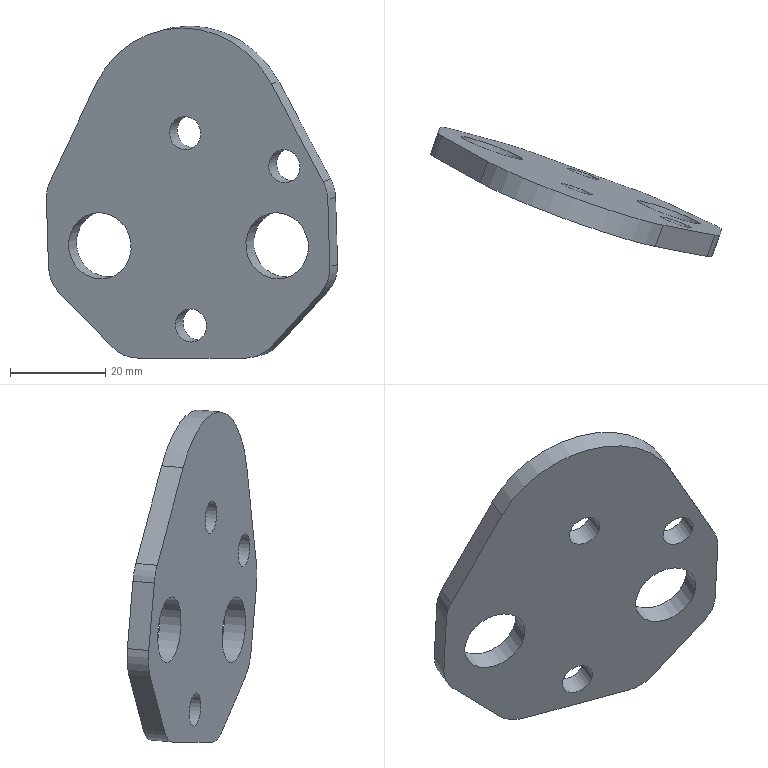Part | NX | features solid 2 | 1 solid | 21 faces | box 61.268 x 27.361 x 69.853 mm | volume 14527 mm3 | cylinder 12 | plane 9 | commonest cylinder face diameters 16 x6 7 x3 14 x2 44.4 x1
STEP:
#1=CARTESIAN_POINT('',(-625.359,149.029,-55.58));
#2=VERTEX_POINT('',#1);
#3=CARTESIAN_POINT('',(-615.065,144.233,-44.309));
#4=VERTEX_POINT('',#3);
#5=CARTESIAN_POINT('',(-627.491,150.023,-57.914));
#6=DIRECTION('',(0.6434,-0.2998,0.7044));
#7=VECTOR('',#6,1000.);
#8=LINE('',#5,#7);
#9=EDGE_CURVE('',#2,#4,#8,.T.);
#10=ORIENTED_EDGE('',*,*,#9,.T.);
#11=CARTESIAN_POINT('',(-616.7,139.74,-44.727));
#12=VERTEX_POINT('',#11);
#13=CARTESIAN_POINT('',(-615.065,144.233,-44.309));
#14=DIRECTION('',(-0.3407,-0.9361,-0.08716));
#15=VECTOR('',#14,1000.);
#16=LINE('',#13,#15);
#17=EDGE_CURVE('',#4,#12,#16,.T.);
#18=ORIENTED_EDGE('',*,*,#17,.T.);
#19=CARTESIAN_POINT('',(-626.994,144.536,-55.998));
#20=VERTEX_POINT('',#19);
#21=CARTESIAN_POINT('',(-629.126,145.529,-58.332));
#22=DIRECTION('',(0.6434,-0.2998,0.7044));
#23=VECTOR('',#22,1000.);
#24=LINE('',#21,#23);
#25=EDGE_CURVE('',#20,#12,#24,.T.);
#26=ORIENTED_EDGE('',*,*,#25,.F.);
#27=CARTESIAN_POINT('',(-625.359,149.029,-55.58));
#28=DIRECTION('',(-0.3407,-0.9361,-0.08716));
#29=VECTOR('',#28,1000.);
#30=LINE('',#27,#29);
#31=EDGE_CURVE('',#20,#2,#30,.F.);
#32=ORIENTED_EDGE('',*,*,#31,.T.);
#33=EDGE_LOOP('',(#10,#18,#26,#32));
#34=FACE_BOUND('',#33,.T.);
#35=CARTESIAN_POINT('',(-627.491,150.023,-57.914));
#36=DIRECTION('',(0.6855,-0.1839,-0.7044));
#37=DIRECTION('',(-0.6434,0.2998,-0.7044));
#38=AXIS2_PLACEMENT_3D('',#35,#36,#37);
#39=PLANE('',#38);
#40=ADVANCED_FACE('',(#34),#39,.T.);
#41=CARTESIAN_POINT('',(-613.032,142.969,-38.674));
#42=VERTEX_POINT('',#41);
#43=CARTESIAN_POINT('',(-613.456,141.803,-24.492));
#44=VERTEX_POINT('',#43);
#45=CARTESIAN_POINT('',(-612.933,143.24,-41.975));
#46=DIRECTION('',(-0.02981,-0.0819,0.9962));
#47=VECTOR('',#46,1000.);
#48=LINE('',#45,#47);
#49=EDGE_CURVE('',#42,#44,#48,.T.);
#50=ORIENTED_EDGE('',*,*,#49,.T.);
#51=CARTESIAN_POINT('',(-615.091,137.309,-24.91));
#52=VERTEX_POINT('',#51);
#53=CARTESIAN_POINT('',(-613.456,141.803,-24.492));
#54=DIRECTION('',(-0.3407,-0.9361,-0.08716));
#55=VECTOR('',#54,1000.);
#56=LINE('',#53,#55);
#57=EDGE_CURVE('',#44,#52,#56,.T.);
#58=ORIENTED_EDGE('',*,*,#57,.T.);
#59=CARTESIAN_POINT('',(-614.667,138.475,-39.092));
#60=VERTEX_POINT('',#59);
#61=CARTESIAN_POINT('',(-614.568,138.747,-42.393));
#62=DIRECTION('',(-0.02981,-0.0819,0.9962));
#63=VECTOR('',#62,1000.);
#64=LINE('',#61,#63);
#65=EDGE_CURVE('',#60,#52,#64,.T.);
#66=ORIENTED_EDGE('',*,*,#65,.F.);
#67=CARTESIAN_POINT('',(-613.032,142.969,-38.674));
#68=DIRECTION('',(-0.3407,-0.9361,-0.08716));
#69=VECTOR('',#68,1000.);
#70=LINE('',#67,#69);
#71=EDGE_CURVE('',#60,#42,#70,.F.);
#72=ORIENTED_EDGE('',*,*,#71,.T.);
#73=EDGE_LOOP('',(#50,#58,#66,#72));
#74=FACE_BOUND('',#73,.T.);
#75=CARTESIAN_POINT('',(-612.933,143.24,-41.975));
#76=DIRECTION('',(0.9397,-0.342,0.));
#77=DIRECTION('',(0.3407,0.9361,0.08716));
#78=AXIS2_PLACEMENT_3D('',#75,#76,#77);
#79=PLANE('',#78);
#80=ADVANCED_FACE('',(#74),#79,.T.);
#81=CARTESIAN_POINT('',(-616.083,137.322,-21.169));
#82=VERTEX_POINT('',#81);
#83=CARTESIAN_POINT('',(-626.999,139.383,-0.6305));
#84=VERTEX_POINT('',#83);
#85=CARTESIAN_POINT('',(-615.151,137.146,-22.923));
#86=DIRECTION('',(-0.4675,0.08826,0.8796));
#87=VECTOR('',#86,1000.);
#88=LINE('',#85,#87);
#89=EDGE_CURVE('',#82,#84,#88,.T.);
#90=ORIENTED_EDGE('',*,*,#89,.F.);
#91=CARTESIAN_POINT('',(-614.448,141.815,-20.751));
#92=VERTEX_POINT('',#91);
#93=CARTESIAN_POINT('',(-614.448,141.815,-20.751));
#94=DIRECTION('',(-0.3407,-0.9361,-0.08716));
#95=VECTOR('',#94,1000.);
#96=LINE('',#93,#95);
#97=EDGE_CURVE('',#82,#92,#96,.F.);
#98=ORIENTED_EDGE('',*,*,#97,.T.);
#99=CARTESIAN_POINT('',(-625.363,143.876,-0.2122));
#100=VERTEX_POINT('',#99);
#101=CARTESIAN_POINT('',(-613.515,141.639,-22.505));
#102=DIRECTION('',(-0.4675,0.08826,0.8796));
#103=VECTOR('',#102,1000.);
#104=LINE('',#101,#103);
#105=EDGE_CURVE('',#92,#100,#104,.T.);
#106=ORIENTED_EDGE('',*,*,#105,.T.);
#107=CARTESIAN_POINT('',(-625.363,143.876,-0.2122));
#108=DIRECTION('',(-0.3407,-0.9361,-0.08716));
#109=VECTOR('',#108,1000.);
#110=LINE('',#107,#109);
#111=EDGE_CURVE('',#100,#84,#110,.T.);
#112=ORIENTED_EDGE('',*,*,#111,.T.);
#113=EDGE_LOOP('',(#90,#98,#106,#112));
#114=FACE_BOUND('',#113,.T.);
#115=CARTESIAN_POINT('',(-613.515,141.639,-22.505));
#116=DIRECTION('',(0.8157,-0.3404,0.4677));
#117=DIRECTION('',(0.4675,-0.08826,-0.8796));
#118=AXIS2_PLACEMENT_3D('',#115,#116,#117);
#119=PLANE('',#118);
#120=ADVANCED_FACE('',(#114),#119,.T.);
#121=CARTESIAN_POINT('',(-663.838,152.791,-0.6305));
#122=VERTEX_POINT('',#121);
#123=CARTESIAN_POINT('',(-645.108,146.94,-11.013));
#124=DIRECTION('',(0.3407,0.9361,0.08716));
#125=DIRECTION('',(-0.02981,-0.0819,0.9962));
#126=AXIS2_PLACEMENT_3D('',#123,#124,#125);
#127=CIRCLE('',#126,22.2);
#128=EDGE_CURVE('',#122,#84,#127,.T.);
#129=ORIENTED_EDGE('',*,*,#128,.T.);
#130=ORIENTED_EDGE('',*,*,#111,.F.);
#131=CARTESIAN_POINT('',(-662.202,157.284,-0.2122));
#132=VERTEX_POINT('',#131);
#133=CARTESIAN_POINT('',(-643.472,151.434,-10.595));
#134=DIRECTION('',(0.3407,0.9361,0.08716));
#135=DIRECTION('',(-0.02981,-0.0819,0.9962));
#136=AXIS2_PLACEMENT_3D('',#133,#134,#135);
#137=CIRCLE('',#136,22.2);
#138=EDGE_CURVE('',#132,#100,#137,.T.);
#139=ORIENTED_EDGE('',*,*,#138,.F.);
#140=CARTESIAN_POINT('',(-662.202,157.284,-0.2122));
#141=DIRECTION('',(-0.3407,-0.9361,-0.08716));
#142=VECTOR('',#141,1000.);
#143=LINE('',#140,#142);
#144=EDGE_CURVE('',#132,#122,#143,.T.);
#145=ORIENTED_EDGE('',*,*,#144,.T.);
#146=EDGE_LOOP('',(#129,#130,#139,#145));
#147=FACE_BOUND('',#146,.T.);
#148=CARTESIAN_POINT('',(-643.472,151.434,-10.595));
#149=DIRECTION('',(-0.3407,-0.9361,-0.08716));
#150=DIRECTION('',(0.02981,0.0819,-0.9962));
#151=AXIS2_PLACEMENT_3D('',#148,#149,#150);
#152=CYLINDRICAL_SURFACE('',#151,22.2);
#153=ADVANCED_FACE('',(#147),#152,.T.);
#154=CARTESIAN_POINT('',(-671.889,162.722,-20.751));
#155=VERTEX_POINT('',#154);
#156=CARTESIAN_POINT('',(-672.716,163.187,-22.505));
#157=DIRECTION('',(0.4148,-0.2329,0.8796));
#158=VECTOR('',#157,1000.);
#159=LINE('',#156,#158);
#160=EDGE_CURVE('',#155,#132,#159,.T.);
#161=ORIENTED_EDGE('',*,*,#160,.F.);
#162=CARTESIAN_POINT('',(-673.524,158.229,-21.169));
#163=VERTEX_POINT('',#162);
#164=CARTESIAN_POINT('',(-671.889,162.722,-20.751));
#165=DIRECTION('',(-0.3407,-0.9361,-0.08716));
#166=VECTOR('',#165,1000.);
#167=LINE('',#164,#166);
#168=EDGE_CURVE('',#155,#163,#167,.T.);
#169=ORIENTED_EDGE('',*,*,#168,.T.);
#170=CARTESIAN_POINT('',(-674.351,158.693,-22.923));
#171=DIRECTION('',(0.4148,-0.2329,0.8796));
#172=VECTOR('',#171,1000.);
#173=LINE('',#170,#172);
#174=EDGE_CURVE('',#163,#122,#173,.T.);
#175=ORIENTED_EDGE('',*,*,#174,.T.);
#176=ORIENTED_EDGE('',*,*,#144,.F.);
#177=EDGE_LOOP('',(#161,#169,#175,#176));
#178=FACE_BOUND('',#177,.T.);
#179=CARTESIAN_POINT('',(-672.716,163.187,-22.505));
#180=DIRECTION('',(0.8437,-0.2635,-0.4677));
#181=DIRECTION('',(-0.4148,0.2329,-0.8796));
#182=AXIS2_PLACEMENT_3D('',#179,#180,#181);
#183=PLANE('',#182);
#184=ADVANCED_FACE('',(#178),#183,.F.);
#185=CARTESIAN_POINT('',(-672.232,164.516,-38.674));
#186=VERTEX_POINT('',#185);
#187=CARTESIAN_POINT('',(-672.657,163.35,-24.492));
#188=VERTEX_POINT('',#187);
#189=CARTESIAN_POINT('',(-672.133,164.787,-41.975));
#190=DIRECTION('',(-0.02981,-0.0819,0.9962));
#191=VECTOR('',#190,1000.);
#192=LINE('',#189,#191);
#193=EDGE_CURVE('',#186,#188,#192,.T.);
#194=ORIENTED_EDGE('',*,*,#193,.F.);
#195=CARTESIAN_POINT('',(-673.868,160.022,-39.092));
#196=VERTEX_POINT('',#195);
#197=CARTESIAN_POINT('',(-672.232,164.516,-38.674));
#198=DIRECTION('',(-0.3407,-0.9361,-0.08716));
#199=VECTOR('',#198,1000.);
#200=LINE('',#197,#199);
#201=EDGE_CURVE('',#186,#196,#200,.T.);
#202=ORIENTED_EDGE('',*,*,#201,.T.);
#203=CARTESIAN_POINT('',(-674.292,158.857,-24.91));
#204=VERTEX_POINT('',#203);
#205=CARTESIAN_POINT('',(-673.769,160.294,-42.393));
#206=DIRECTION('',(-0.02981,-0.0819,0.9962));
#207=VECTOR('',#206,1000.);
#208=LINE('',#205,#207);
#209=EDGE_CURVE('',#196,#204,#208,.T.);
#210=ORIENTED_EDGE('',*,*,#209,.T.);
#211=CARTESIAN_POINT('',(-672.657,163.35,-24.492));
#212=DIRECTION('',(-0.3407,-0.9361,-0.08716));
#213=VECTOR('',#212,1000.);
#214=LINE('',#211,#213);
#215=EDGE_CURVE('',#204,#188,#214,.F.);
#216=ORIENTED_EDGE('',*,*,#215,.T.);
#217=EDGE_LOOP('',(#194,#202,#210,#216));
#218=FACE_BOUND('',#217,.T.);
#219=CARTESIAN_POINT('',(-672.133,164.787,-41.975));
#220=DIRECTION('',(0.9397,-0.342,0.));
#221=DIRECTION('',(0.3407,0.9361,0.08716));
#222=AXIS2_PLACEMENT_3D('',#219,#220,#221);
#223=PLANE('',#222);
#224=ADVANCED_FACE('',(#218),#223,.F.);
#225=CARTESIAN_POINT('',(-658.893,161.235,-55.58));
#226=VERTEX_POINT('',#225);
#227=CARTESIAN_POINT('',(-669.862,164.178,-44.309));
#228=VERTEX_POINT('',#227);
#229=CARTESIAN_POINT('',(-656.621,160.625,-57.914));
#230=DIRECTION('',(-0.6855,0.1839,0.7044));
#231=VECTOR('',#230,1000.);
#232=LINE('',#229,#231);
#233=EDGE_CURVE('',#226,#228,#232,.T.);
#234=ORIENTED_EDGE('',*,*,#233,.F.);
#235=CARTESIAN_POINT('',(-660.529,156.741,-55.998));
#236=VERTEX_POINT('',#235);
#237=CARTESIAN_POINT('',(-660.529,156.741,-55.998));
#238=DIRECTION('',(-0.3407,-0.9361,-0.08716));
#239=VECTOR('',#238,1000.);
#240=LINE('',#237,#239);
#241=EDGE_CURVE('',#226,#236,#240,.T.);
#242=ORIENTED_EDGE('',*,*,#241,.T.);
#243=CARTESIAN_POINT('',(-671.497,159.684,-44.727));
#244=VERTEX_POINT('',#243);
#245=CARTESIAN_POINT('',(-658.257,156.132,-58.332));
#246=DIRECTION('',(-0.6855,0.1839,0.7044));
#247=VECTOR('',#246,1000.);
#248=LINE('',#245,#247);
#249=EDGE_CURVE('',#236,#244,#248,.T.);
#250=ORIENTED_EDGE('',*,*,#249,.T.);
#251=CARTESIAN_POINT('',(-669.862,164.178,-44.309));
#252=DIRECTION('',(-0.3407,-0.9361,-0.08716));
#253=VECTOR('',#252,1000.);
#254=LINE('',#251,#253);
#255=EDGE_CURVE('',#244,#228,#254,.F.);
#256=ORIENTED_EDGE('',*,*,#255,.T.);
#257=EDGE_LOOP('',(#234,#242,#250,#256));
#258=FACE_BOUND('',#257,.T.);
#259=CARTESIAN_POINT('',(-656.621,160.625,-57.914));
#260=DIRECTION('',(0.6434,-0.2998,0.7044));
#261=DIRECTION('',(0.6855,-0.1839,-0.7044));
#262=AXIS2_PLACEMENT_3D('',#259,#260,#261);
#263=PLANE('',#262);
#264=ADVANCED_FACE('',(#258),#263,.F.);
#265=CARTESIAN_POINT('',(-653.508,159.492,-57.914));
#266=VERTEX_POINT('',#265);
#267=CARTESIAN_POINT('',(-630.605,151.156,-57.914));
#268=VERTEX_POINT('',#267);
#269=CARTESIAN_POINT('',(-656.621,160.625,-57.914));
#270=DIRECTION('',(0.9397,-0.342,0.));
#271=VECTOR('',#270,1000.);
#272=LINE('',#269,#271);
#273=EDGE_CURVE('',#266,#268,#272,.T.);
#274=ORIENTED_EDGE('',*,*,#273,.T.);
#275=CARTESIAN_POINT('',(-632.24,146.663,-58.332));
#276=VERTEX_POINT('',#275);
#277=CARTESIAN_POINT('',(-630.605,151.156,-57.914));
#278=DIRECTION('',(-0.3407,-0.9361,-0.08716));
#279=VECTOR('',#278,1000.);
#280=LINE('',#277,#279);
#281=EDGE_CURVE('',#268,#276,#280,.T.);
#282=ORIENTED_EDGE('',*,*,#281,.T.);
#283=CARTESIAN_POINT('',(-655.143,154.999,-58.332));
#284=VERTEX_POINT('',#283);
#285=CARTESIAN_POINT('',(-658.257,156.132,-58.332));
#286=DIRECTION('',(0.9397,-0.342,0.));
#287=VECTOR('',#286,1000.);
#288=LINE('',#285,#287);
#289=EDGE_CURVE('',#284,#276,#288,.T.);
#290=ORIENTED_EDGE('',*,*,#289,.F.);
#291=CARTESIAN_POINT('',(-653.508,159.492,-57.914));
#292=DIRECTION('',(-0.3407,-0.9361,-0.08716));
#293=VECTOR('',#292,1000.);
#294=LINE('',#291,#293);
#295=EDGE_CURVE('',#284,#266,#294,.F.);
#296=ORIENTED_EDGE('',*,*,#295,.T.);
#297=EDGE_LOOP('',(#274,#282,#290,#296));
#298=FACE_BOUND('',#297,.T.);
#299=CARTESIAN_POINT('',(-656.621,160.625,-57.914));
#300=DIRECTION('',(0.02981,0.0819,-0.9962));
#301=DIRECTION('',(0.3407,0.9361,0.08716));
#302=AXIS2_PLACEMENT_3D('',#299,#300,#301);
#303=PLANE('',#302);
#304=ADVANCED_FACE('',(#298),#303,.T.);
#305=CARTESIAN_POINT('',(-661.197,160.742,-41.278));
#306=VERTEX_POINT('',#305);
#307=CARTESIAN_POINT('',(-661.406,160.169,-34.304));
#308=DIRECTION('',(-0.3407,-0.9361,-0.08716));
#309=DIRECTION('',(0.02981,0.0819,-0.9962));
#310=AXIS2_PLACEMENT_3D('',#307,#308,#309);
#311=CIRCLE('',#310,7.);
#312=EDGE_CURVE('',#306,#306,#311,.T.);
#313=ORIENTED_EDGE('',*,*,#312,.T.);
#314=EDGE_LOOP('',(#313));
#315=FACE_BOUND('',#314,.T.);
#316=CARTESIAN_POINT('',(-623.91,147.171,-41.278));
#317=VERTEX_POINT('',#316);
#318=CARTESIAN_POINT('',(-624.119,146.597,-34.304));
#319=DIRECTION('',(-0.3407,-0.9361,-0.08716));
#320=DIRECTION('',(0.02981,0.0819,-0.9962));
#321=AXIS2_PLACEMENT_3D('',#318,#319,#320);
#322=CIRCLE('',#321,7.);
#323=EDGE_CURVE('',#317,#317,#322,.T.);
#324=ORIENTED_EDGE('',*,*,#323,.T.);
#325=EDGE_LOOP('',(#324));
#326=FACE_BOUND('',#325,.T.);
#327=CARTESIAN_POINT('',(-622.486,144.769,-21.055));
#328=VERTEX_POINT('',#327);
#329=CARTESIAN_POINT('',(-622.59,144.483,-17.568));
#330=DIRECTION('',(-0.3407,-0.9361,-0.08716));
#331=DIRECTION('',(0.02981,0.0819,-0.9962));
#332=AXIS2_PLACEMENT_3D('',#329,#330,#331);
#333=CIRCLE('',#332,3.5);
#334=EDGE_CURVE('',#328,#328,#333,.T.);
#335=ORIENTED_EDGE('',*,*,#334,.T.);
#336=EDGE_LOOP('',(#335));
#337=FACE_BOUND('',#336,.T.);
#338=CARTESIAN_POINT('',(-642.156,155.049,-54.567));
#339=VERTEX_POINT('',#338);
#340=CARTESIAN_POINT('',(-642.261,154.762,-51.08));
#341=DIRECTION('',(-0.3407,-0.9361,-0.08716));
#342=DIRECTION('',(0.02981,0.0819,-0.9962));
#343=AXIS2_PLACEMENT_3D('',#340,#341,#342);
#344=CIRCLE('',#343,3.5);
#345=EDGE_CURVE('',#339,#339,#344,.T.);
#346=ORIENTED_EDGE('',*,*,#345,.T.);
#347=EDGE_LOOP('',(#346));
#348=FACE_BOUND('',#347,.T.);
#349=CARTESIAN_POINT('',(-643.368,151.72,-14.081));
#350=VERTEX_POINT('',#349);
#351=CARTESIAN_POINT('',(-643.472,151.434,-10.595));
#352=DIRECTION('',(-0.3407,-0.9361,-0.08716));
#353=DIRECTION('',(0.02981,0.0819,-0.9962));
#354=AXIS2_PLACEMENT_3D('',#351,#352,#353);
#355=CIRCLE('',#354,3.5);
#356=EDGE_CURVE('',#350,#350,#355,.T.);
#357=ORIENTED_EDGE('',*,*,#356,.T.);
#358=EDGE_LOOP('',(#357));
#359=FACE_BOUND('',#358,.T.);
#360=ORIENTED_EDGE('',*,*,#105,.F.);
#361=CARTESIAN_POINT('',(-620.973,144.539,-24.492));
#362=DIRECTION('',(0.3407,0.9361,0.08716));
#363=DIRECTION('',(-0.02981,-0.0819,0.9962));
#364=AXIS2_PLACEMENT_3D('',#361,#362,#363);
#365=CIRCLE('',#364,8.);
#366=EDGE_CURVE('',#92,#44,#365,.T.);
#367=ORIENTED_EDGE('',*,*,#366,.T.);
#368=ORIENTED_EDGE('',*,*,#49,.F.);
#369=CARTESIAN_POINT('',(-620.549,145.705,-38.674));
#370=DIRECTION('',(0.3407,0.9361,0.08716));
#371=DIRECTION('',(-0.02981,-0.0819,0.9962));
#372=AXIS2_PLACEMENT_3D('',#369,#370,#371);
#373=CIRCLE('',#372,8.);
#374=EDGE_CURVE('',#42,#4,#373,.T.);
#375=ORIENTED_EDGE('',*,*,#374,.T.);
#376=ORIENTED_EDGE('',*,*,#9,.F.);
#377=CARTESIAN_POINT('',(-630.843,150.501,-49.944));
#378=DIRECTION('',(0.3407,0.9361,0.08716));
#379=DIRECTION('',(-0.02981,-0.0819,0.9962));
#380=AXIS2_PLACEMENT_3D('',#377,#378,#379);
#381=CIRCLE('',#380,8.);
#382=EDGE_CURVE('',#2,#268,#381,.T.);
#383=ORIENTED_EDGE('',*,*,#382,.T.);
#384=ORIENTED_EDGE('',*,*,#273,.F.);
#385=CARTESIAN_POINT('',(-653.746,158.837,-49.944));
#386=DIRECTION('',(0.3407,0.9361,0.08716));
#387=DIRECTION('',(-0.02981,-0.0819,0.9962));
#388=AXIS2_PLACEMENT_3D('',#385,#386,#387);
#389=CIRCLE('',#388,8.);
#390=EDGE_CURVE('',#266,#226,#389,.T.);
#391=ORIENTED_EDGE('',*,*,#390,.T.);
#392=ORIENTED_EDGE('',*,*,#233,.T.);
#393=CARTESIAN_POINT('',(-664.715,161.78,-38.674));
#394=DIRECTION('',(0.3407,0.9361,0.08716));
#395=DIRECTION('',(-0.02981,-0.0819,0.9962));
#396=AXIS2_PLACEMENT_3D('',#393,#394,#395);
#397=CIRCLE('',#396,8.);
#398=EDGE_CURVE('',#228,#186,#397,.T.);
#399=ORIENTED_EDGE('',*,*,#398,.T.);
#400=ORIENTED_EDGE('',*,*,#193,.T.);
#401=CARTESIAN_POINT('',(-665.139,160.614,-24.492));
#402=DIRECTION('',(0.3407,0.9361,0.08716));
#403=DIRECTION('',(-0.02981,-0.0819,0.9962));
#404=AXIS2_PLACEMENT_3D('',#401,#402,#403);
#405=CIRCLE('',#404,8.);
#406=EDGE_CURVE('',#188,#155,#405,.T.);
#407=ORIENTED_EDGE('',*,*,#406,.T.);
#408=ORIENTED_EDGE('',*,*,#160,.T.);
#409=ORIENTED_EDGE('',*,*,#138,.T.);
#410=EDGE_LOOP('',(#360,#367,#368,#375,#376,#383,#384,#391,#392,#399,#400,#407,#408,#409));
#411=FACE_BOUND('',#410,.T.);
#412=CARTESIAN_POINT('',(-643.472,151.434,-10.595));
#413=DIRECTION('',(0.3407,0.9361,0.08716));
#414=DIRECTION('',(-0.02981,-0.0819,0.9962));
#415=AXIS2_PLACEMENT_3D('',#412,#413,#414);
#416=PLANE('',#415);
#417=ADVANCED_FACE('',(#315,#326,#337,#348,#359,#411),#416,.T.);
#418=CARTESIAN_POINT('',(-663.25,155.102,-27.749));
#419=VERTEX_POINT('',#418);
#420=CARTESIAN_POINT('',(-663.042,155.675,-34.723));
#421=DIRECTION('',(0.3407,0.9361,0.08716));
#422=DIRECTION('',(-0.02981,-0.0819,0.9962));
#423=AXIS2_PLACEMENT_3D('',#420,#421,#422);
#424=CIRCLE('',#423,7.);
#425=EDGE_CURVE('',#419,#419,#424,.T.);
#426=ORIENTED_EDGE('',*,*,#425,.T.);
#427=EDGE_LOOP('',(#426));
#428=FACE_BOUND('',#427,.T.);
#429=CARTESIAN_POINT('',(-625.963,141.531,-27.749));
#430=VERTEX_POINT('',#429);
#431=CARTESIAN_POINT('',(-625.755,142.104,-34.723));
#432=DIRECTION('',(0.3407,0.9361,0.08716));
#433=DIRECTION('',(-0.02981,-0.0819,0.9962));
#434=AXIS2_PLACEMENT_3D('',#431,#432,#433);
#435=CIRCLE('',#434,7.);
#436=EDGE_CURVE('',#430,#430,#435,.T.);
#437=ORIENTED_EDGE('',*,*,#436,.T.);
#438=EDGE_LOOP('',(#437));
#439=FACE_BOUND('',#438,.T.);
#440=CARTESIAN_POINT('',(-624.33,139.703,-14.5));
#441=VERTEX_POINT('',#440);
#442=CARTESIAN_POINT('',(-624.226,139.989,-17.986));
#443=DIRECTION('',(0.3407,0.9361,0.08716));
#444=DIRECTION('',(-0.02981,-0.0819,0.9962));
#445=AXIS2_PLACEMENT_3D('',#442,#443,#444);
#446=CIRCLE('',#445,3.5);
#447=EDGE_CURVE('',#441,#441,#446,.T.);
#448=ORIENTED_EDGE('',*,*,#447,.T.);
#449=EDGE_LOOP('',(#448));
#450=FACE_BOUND('',#449,.T.);
#451=CARTESIAN_POINT('',(-644.,149.982,-48.012));
#452=VERTEX_POINT('',#451);
#453=CARTESIAN_POINT('',(-643.896,150.269,-51.498));
#454=DIRECTION('',(0.3407,0.9361,0.08716));
#455=DIRECTION('',(-0.02981,-0.0819,0.9962));
#456=AXIS2_PLACEMENT_3D('',#453,#454,#455);
#457=CIRCLE('',#456,3.5);
#458=EDGE_CURVE('',#452,#452,#457,.T.);
#459=ORIENTED_EDGE('',*,*,#458,.T.);
#460=EDGE_LOOP('',(#459));
#461=FACE_BOUND('',#460,.T.);
#462=CARTESIAN_POINT('',(-645.212,146.654,-7.526));
#463=VERTEX_POINT('',#462);
#464=CARTESIAN_POINT('',(-645.108,146.94,-11.013));
#465=DIRECTION('',(0.3407,0.9361,0.08716));
#466=DIRECTION('',(-0.02981,-0.0819,0.9962));
#467=AXIS2_PLACEMENT_3D('',#464,#465,#466);
#468=CIRCLE('',#467,3.5);
#469=EDGE_CURVE('',#463,#463,#468,.T.);
#470=ORIENTED_EDGE('',*,*,#469,.T.);
#471=EDGE_LOOP('',(#470));
#472=FACE_BOUND('',#471,.T.);
#473=ORIENTED_EDGE('',*,*,#65,.T.);
#474=CARTESIAN_POINT('',(-622.609,140.045,-24.91));
#475=DIRECTION('',(0.3407,0.9361,0.08716));
#476=DIRECTION('',(-0.02981,-0.0819,0.9962));
#477=AXIS2_PLACEMENT_3D('',#474,#475,#476);
#478=CIRCLE('',#477,8.);
#479=EDGE_CURVE('',#52,#82,#478,.F.);
#480=ORIENTED_EDGE('',*,*,#479,.T.);
#481=ORIENTED_EDGE('',*,*,#89,.T.);
#482=ORIENTED_EDGE('',*,*,#128,.F.);
#483=ORIENTED_EDGE('',*,*,#174,.F.);
#484=CARTESIAN_POINT('',(-666.774,156.12,-24.91));
#485=DIRECTION('',(0.3407,0.9361,0.08716));
#486=DIRECTION('',(-0.02981,-0.0819,0.9962));
#487=AXIS2_PLACEMENT_3D('',#484,#485,#486);
#488=CIRCLE('',#487,8.);
#489=EDGE_CURVE('',#163,#204,#488,.F.);
#490=ORIENTED_EDGE('',*,*,#489,.T.);
#491=ORIENTED_EDGE('',*,*,#209,.F.);
#492=CARTESIAN_POINT('',(-666.35,157.286,-39.092));
#493=DIRECTION('',(0.3407,0.9361,0.08716));
#494=DIRECTION('',(-0.02981,-0.0819,0.9962));
#495=AXIS2_PLACEMENT_3D('',#492,#493,#494);
#496=CIRCLE('',#495,8.);
#497=EDGE_CURVE('',#196,#244,#496,.F.);
#498=ORIENTED_EDGE('',*,*,#497,.T.);
#499=ORIENTED_EDGE('',*,*,#249,.F.);
#500=CARTESIAN_POINT('',(-655.381,154.343,-50.363));
#501=DIRECTION('',(0.3407,0.9361,0.08716));
#502=DIRECTION('',(-0.02981,-0.0819,0.9962));
#503=AXIS2_PLACEMENT_3D('',#500,#501,#502);
#504=CIRCLE('',#503,8.);
#505=EDGE_CURVE('',#236,#284,#504,.F.);
#506=ORIENTED_EDGE('',*,*,#505,.T.);
#507=ORIENTED_EDGE('',*,*,#289,.T.);
#508=CARTESIAN_POINT('',(-632.479,146.007,-50.363));
#509=DIRECTION('',(0.3407,0.9361,0.08716));
#510=DIRECTION('',(-0.02981,-0.0819,0.9962));
#511=AXIS2_PLACEMENT_3D('',#508,#509,#510);
#512=CIRCLE('',#511,8.);
#513=EDGE_CURVE('',#276,#20,#512,.F.);
#514=ORIENTED_EDGE('',*,*,#513,.T.);
#515=ORIENTED_EDGE('',*,*,#25,.T.);
#516=CARTESIAN_POINT('',(-622.185,141.211,-39.092));
#517=DIRECTION('',(0.3407,0.9361,0.08716));
#518=DIRECTION('',(-0.02981,-0.0819,0.9962));
#519=AXIS2_PLACEMENT_3D('',#516,#517,#518);
#520=CIRCLE('',#519,8.);
#521=EDGE_CURVE('',#12,#60,#520,.F.);
#522=ORIENTED_EDGE('',*,*,#521,.T.);
#523=EDGE_LOOP('',(#473,#480,#481,#482,#483,#490,#491,#498,#499,#506,#507,#514,#515,#522));
#524=FACE_BOUND('',#523,.T.);
#525=CARTESIAN_POINT('',(-645.108,146.94,-11.013));
#526=DIRECTION('',(0.3407,0.9361,0.08716));
#527=DIRECTION('',(-0.02981,-0.0819,0.9962));
#528=AXIS2_PLACEMENT_3D('',#525,#526,#527);
#529=PLANE('',#528);
#530=ADVANCED_FACE('',(#428,#439,#450,#461,#472,#524),#529,.F.);
#531=ORIENTED_EDGE('',*,*,#356,.F.);
#532=EDGE_LOOP('',(#531));
#533=FACE_BOUND('',#532,.T.);
#534=ORIENTED_EDGE('',*,*,#469,.F.);
#535=EDGE_LOOP('',(#534));
#536=FACE_BOUND('',#535,.T.);
#537=CARTESIAN_POINT('',(-645.108,146.94,-11.013));
#538=DIRECTION('',(0.3407,0.9361,0.08716));
#539=DIRECTION('',(-0.02981,-0.0819,0.9962));
#540=AXIS2_PLACEMENT_3D('',#537,#538,#539);
#541=CYLINDRICAL_SURFACE('',#540,3.5);
#542=ADVANCED_FACE('',(#533,#536),#541,.F.);
#543=ORIENTED_EDGE('',*,*,#345,.F.);
#544=EDGE_LOOP('',(#543));
#545=FACE_BOUND('',#544,.T.);
#546=ORIENTED_EDGE('',*,*,#458,.F.);
#547=EDGE_LOOP('',(#546));
#548=FACE_BOUND('',#547,.T.);
#549=CARTESIAN_POINT('',(-643.896,150.269,-51.498));
#550=DIRECTION('',(0.3407,0.9361,0.08716));
#551=DIRECTION('',(-0.02981,-0.0819,0.9962));
#552=AXIS2_PLACEMENT_3D('',#549,#550,#551);
#553=CYLINDRICAL_SURFACE('',#552,3.5);
#554=ADVANCED_FACE('',(#545,#548),#553,.F.);
#555=ORIENTED_EDGE('',*,*,#334,.F.);
#556=EDGE_LOOP('',(#555));
#557=FACE_BOUND('',#556,.T.);
#558=ORIENTED_EDGE('',*,*,#447,.F.);
#559=EDGE_LOOP('',(#558));
#560=FACE_BOUND('',#559,.T.);
#561=CARTESIAN_POINT('',(-624.226,139.989,-17.986));
#562=DIRECTION('',(0.3407,0.9361,0.08716));
#563=DIRECTION('',(-0.02981,-0.0819,0.9962));
#564=AXIS2_PLACEMENT_3D('',#561,#562,#563);
#565=CYLINDRICAL_SURFACE('',#564,3.5);
#566=ADVANCED_FACE('',(#557,#560),#565,.F.);
#567=ORIENTED_EDGE('',*,*,#323,.F.);
#568=EDGE_LOOP('',(#567));
#569=FACE_BOUND('',#568,.T.);
#570=ORIENTED_EDGE('',*,*,#436,.F.);
#571=EDGE_LOOP('',(#570));
#572=FACE_BOUND('',#571,.T.);
#573=CARTESIAN_POINT('',(-625.755,142.104,-34.723));
#574=DIRECTION('',(0.3407,0.9361,0.08716));
#575=DIRECTION('',(-0.02981,-0.0819,0.9962));
#576=AXIS2_PLACEMENT_3D('',#573,#574,#575);
#577=CYLINDRICAL_SURFACE('',#576,7.);
#578=ADVANCED_FACE('',(#569,#572),#577,.F.);
#579=ORIENTED_EDGE('',*,*,#312,.F.);
#580=EDGE_LOOP('',(#579));
#581=FACE_BOUND('',#580,.T.);
#582=ORIENTED_EDGE('',*,*,#425,.F.);
#583=EDGE_LOOP('',(#582));
#584=FACE_BOUND('',#583,.T.);
#585=CARTESIAN_POINT('',(-663.042,155.675,-34.723));
#586=DIRECTION('',(0.3407,0.9361,0.08716));
#587=DIRECTION('',(-0.02981,-0.0819,0.9962));
#588=AXIS2_PLACEMENT_3D('',#585,#586,#587);
#589=CYLINDRICAL_SURFACE('',#588,7.);
#590=ADVANCED_FACE('',(#581,#584),#589,.F.);
#591=ORIENTED_EDGE('',*,*,#374,.F.);
#592=ORIENTED_EDGE('',*,*,#71,.F.);
#593=ORIENTED_EDGE('',*,*,#521,.F.);
#594=ORIENTED_EDGE('',*,*,#17,.F.);
#595=EDGE_LOOP('',(#591,#592,#593,#594));
#596=FACE_BOUND('',#595,.T.);
#597=CARTESIAN_POINT('',(-620.549,145.705,-38.674));
#598=DIRECTION('',(-0.3407,-0.9361,-0.08716));
#599=DIRECTION('',(0.02981,0.0819,-0.9962));
#600=AXIS2_PLACEMENT_3D('',#597,#598,#599);
#601=CYLINDRICAL_SURFACE('',#600,8.);
#602=ADVANCED_FACE('',(#596),#601,.T.);
#603=ORIENTED_EDGE('',*,*,#382,.F.);
#604=ORIENTED_EDGE('',*,*,#31,.F.);
#605=ORIENTED_EDGE('',*,*,#513,.F.);
#606=ORIENTED_EDGE('',*,*,#281,.F.);
#607=EDGE_LOOP('',(#603,#604,#605,#606));
#608=FACE_BOUND('',#607,.T.);
#609=CARTESIAN_POINT('',(-630.843,150.501,-49.944));
#610=DIRECTION('',(-0.3407,-0.9361,-0.08716));
#611=DIRECTION('',(0.02981,0.0819,-0.9962));
#612=AXIS2_PLACEMENT_3D('',#609,#610,#611);
#613=CYLINDRICAL_SURFACE('',#612,8.);
#614=ADVANCED_FACE('',(#608),#613,.T.);
#615=ORIENTED_EDGE('',*,*,#390,.F.);
#616=ORIENTED_EDGE('',*,*,#295,.F.);
#617=ORIENTED_EDGE('',*,*,#505,.F.);
#618=ORIENTED_EDGE('',*,*,#241,.F.);
#619=EDGE_LOOP('',(#615,#616,#617,#618));
#620=FACE_BOUND('',#619,.T.);
#621=CARTESIAN_POINT('',(-653.746,158.837,-49.944));
#622=DIRECTION('',(0.3407,0.9361,0.08716));
#623=DIRECTION('',(-0.02981,-0.0819,0.9962));
#624=AXIS2_PLACEMENT_3D('',#621,#622,#623);
#625=CYLINDRICAL_SURFACE('',#624,8.);
#626=ADVANCED_FACE('',(#620),#625,.T.);
#627=ORIENTED_EDGE('',*,*,#398,.F.);
#628=ORIENTED_EDGE('',*,*,#255,.F.);
#629=ORIENTED_EDGE('',*,*,#497,.F.);
#630=ORIENTED_EDGE('',*,*,#201,.F.);
#631=EDGE_LOOP('',(#627,#628,#629,#630));
#632=FACE_BOUND('',#631,.T.);
#633=CARTESIAN_POINT('',(-664.715,161.78,-38.674));
#634=DIRECTION('',(-0.3407,-0.9361,-0.08716));
#635=DIRECTION('',(0.02981,0.0819,-0.9962));
#636=AXIS2_PLACEMENT_3D('',#633,#634,#635);
#637=CYLINDRICAL_SURFACE('',#636,8.);
#638=ADVANCED_FACE('',(#632),#637,.T.);
#639=ORIENTED_EDGE('',*,*,#406,.F.);
#640=ORIENTED_EDGE('',*,*,#215,.F.);
#641=ORIENTED_EDGE('',*,*,#489,.F.);
#642=ORIENTED_EDGE('',*,*,#168,.F.);
#643=EDGE_LOOP('',(#639,#640,#641,#642));
#644=FACE_BOUND('',#643,.T.);
#645=CARTESIAN_POINT('',(-665.139,160.614,-24.492));
#646=DIRECTION('',(-0.3407,-0.9361,-0.08716));
#647=DIRECTION('',(0.02981,0.0819,-0.9962));
#648=AXIS2_PLACEMENT_3D('',#645,#646,#647);
#649=CYLINDRICAL_SURFACE('',#648,8.);
#650=ADVANCED_FACE('',(#644),#649,.T.);
#651=ORIENTED_EDGE('',*,*,#366,.F.);
#652=ORIENTED_EDGE('',*,*,#97,.F.);
#653=ORIENTED_EDGE('',*,*,#479,.F.);
#654=ORIENTED_EDGE('',*,*,#57,.F.);
#655=EDGE_LOOP('',(#651,#652,#653,#654));
#656=FACE_BOUND('',#655,.T.);
#657=CARTESIAN_POINT('',(-620.973,144.539,-24.492));
#658=DIRECTION('',(-0.3407,-0.9361,-0.08716));
#659=DIRECTION('',(0.02981,0.0819,-0.9962));
#660=AXIS2_PLACEMENT_3D('',#657,#658,#659);
#661=CYLINDRICAL_SURFACE('',#660,8.);
#662=ADVANCED_FACE('',(#656),#661,.T.);
#663=CLOSED_SHELL('',(#40,#80,#120,#153,#184,#224,#264,#304,#417,#530,#542,#554,#566,#578,#590,#602,#614,#626,#638,#650,#662));
#664=MANIFOLD_SOLID_BREP('',#663);
#665=(LENGTH_UNIT()NAMED_UNIT(*)SI_UNIT(.MILLI.,.METRE.));
#666=UNCERTAINTY_MEASURE_WITH_UNIT(LENGTH_MEASURE(0.00001),#665,'','');
#667=(NAMED_UNIT(*)PLANE_ANGLE_UNIT()SI_UNIT($,.RADIAN.));
#668=(NAMED_UNIT(*)SI_UNIT($,.STERADIAN.)SOLID_ANGLE_UNIT());
#669=(GEOMETRIC_REPRESENTATION_CONTEXT(3)GLOBAL_UNCERTAINTY_ASSIGNED_CONTEXT((#666))GLOBAL_UNIT_ASSIGNED_CONTEXT((#665,#667,#668))REPRESENTATION_CONTEXT('',''));
#670=ADVANCED_BREP_SHAPE_REPRESENTATION('',(#664),#669);